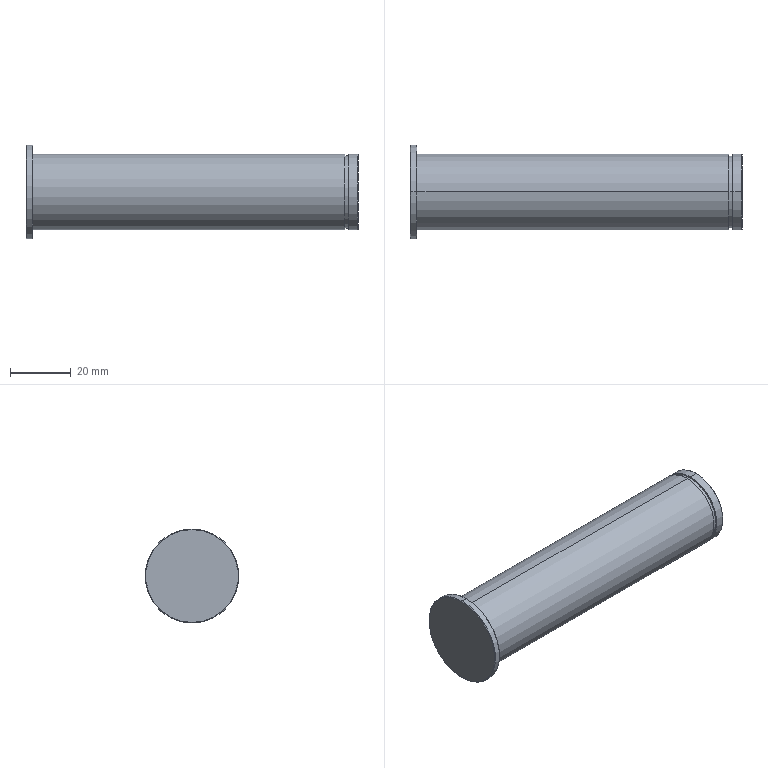Part | STEP file | BT2022003-01-04 Pin shaft A | 1 solid | 19 faces | box 109.5 x 31 x 31 mm | volume 54297 mm3 | cylinder 8 | cone 6 | plane 5 | commonest cylinder face diameters 25 x4 23.9 x2 31 x2
STEP:
#1=CARTESIAN_POINT('',(2.3,0.,-15.3));
#2=VERTEX_POINT('',#1);
#3=CARTESIAN_POINT('',(2.3,0.,15.3));
#4=VERTEX_POINT('',#3);
#5=CARTESIAN_POINT('',(2.3,0.,0.));
#6=DIRECTION('',(1.,0.,0.));
#7=DIRECTION('',(0.,0.,1.));
#8=AXIS2_PLACEMENT_3D('',#5,#6,#7);
#9=CIRCLE('',#8,15.3);
#10=EDGE_CURVE('',#2,#4,#9,.T.);
#11=ORIENTED_EDGE('',*,*,#10,.F.);
#12=CARTESIAN_POINT('',(2.1,0.,-15.5));
#13=VERTEX_POINT('',#12);
#14=CARTESIAN_POINT('',(2.1,0.,-15.5));
#15=DIRECTION('',(-0.7071,0.,-0.7071));
#16=VECTOR('',#15,1000.);
#17=LINE('',#14,#16);
#18=EDGE_CURVE('',#2,#13,#17,.T.);
#19=ORIENTED_EDGE('',*,*,#18,.T.);
#20=CARTESIAN_POINT('',(2.1,0.,15.5));
#21=VERTEX_POINT('',#20);
#22=CARTESIAN_POINT('',(2.1,0.,0.));
#23=DIRECTION('',(-1.,0.,0.));
#24=DIRECTION('',(0.,0.,1.));
#25=AXIS2_PLACEMENT_3D('',#22,#23,#24);
#26=CIRCLE('',#25,15.5);
#27=EDGE_CURVE('',#21,#13,#26,.T.);
#28=ORIENTED_EDGE('',*,*,#27,.F.);
#29=CARTESIAN_POINT('',(2.1,0.,15.5));
#30=DIRECTION('',(-0.7071,0.,0.7071));
#31=VECTOR('',#30,1000.);
#32=LINE('',#29,#31);
#33=EDGE_CURVE('',#4,#21,#32,.T.);
#34=ORIENTED_EDGE('',*,*,#33,.F.);
#35=EDGE_LOOP('',(#11,#19,#28,#34));
#36=FACE_OUTER_BOUND('',#35,.T.);
#37=CARTESIAN_POINT('',(2.1,0.,0.));
#38=DIRECTION('',(-1.,0.,0.));
#39=DIRECTION('',(0.,0.,1.));
#40=AXIS2_PLACEMENT_3D('',#37,#38,#39);
#41=CONICAL_SURFACE('',#40,15.5,0.7854);
#42=ADVANCED_FACE('',(#36),#41,.T.);
#43=CARTESIAN_POINT('',(0.,0.,15.3));
#44=VERTEX_POINT('',#43);
#45=CARTESIAN_POINT('',(0.,0.,-15.3));
#46=VERTEX_POINT('',#45);
#47=CARTESIAN_POINT('',(0.,0.,0.));
#48=DIRECTION('',(-1.,0.,0.));
#49=DIRECTION('',(0.,0.,-1.));
#50=AXIS2_PLACEMENT_3D('',#47,#48,#49);
#51=CIRCLE('',#50,15.3);
#52=EDGE_CURVE('',#44,#46,#51,.T.);
#53=ORIENTED_EDGE('',*,*,#52,.F.);
#54=CARTESIAN_POINT('',(0.2,0.,15.5));
#55=VERTEX_POINT('',#54);
#56=CARTESIAN_POINT('',(0.,0.,15.3));
#57=DIRECTION('',(0.7071,0.,0.7071));
#58=VECTOR('',#57,1000.);
#59=LINE('',#56,#58);
#60=EDGE_CURVE('',#44,#55,#59,.T.);
#61=ORIENTED_EDGE('',*,*,#60,.T.);
#62=CARTESIAN_POINT('',(0.2,0.,-15.5));
#63=VERTEX_POINT('',#62);
#64=CARTESIAN_POINT('',(0.2,0.,0.));
#65=DIRECTION('',(1.,0.,0.));
#66=DIRECTION('',(0.,0.,-1.));
#67=AXIS2_PLACEMENT_3D('',#64,#65,#66);
#68=CIRCLE('',#67,15.5);
#69=EDGE_CURVE('',#63,#55,#68,.T.);
#70=ORIENTED_EDGE('',*,*,#69,.F.);
#71=CARTESIAN_POINT('',(0.,0.,-15.3));
#72=DIRECTION('',(0.7071,0.,-0.7071));
#73=VECTOR('',#72,1000.);
#74=LINE('',#71,#73);
#75=EDGE_CURVE('',#46,#63,#74,.T.);
#76=ORIENTED_EDGE('',*,*,#75,.F.);
#77=EDGE_LOOP('',(#53,#61,#70,#76));
#78=FACE_OUTER_BOUND('',#77,.T.);
#79=CARTESIAN_POINT('',(0.,0.,0.));
#80=DIRECTION('',(1.,0.,0.));
#81=DIRECTION('',(0.,0.,-1.));
#82=AXIS2_PLACEMENT_3D('',#79,#80,#81);
#83=CONICAL_SURFACE('',#82,15.3,0.7854);
#84=ADVANCED_FACE('',(#78),#83,.T.);
#85=CARTESIAN_POINT('',(109.5,0.,-12.3));
#86=VERTEX_POINT('',#85);
#87=CARTESIAN_POINT('',(109.5,0.,12.3));
#88=VERTEX_POINT('',#87);
#89=CARTESIAN_POINT('',(109.5,0.,0.));
#90=DIRECTION('',(1.,0.,0.));
#91=DIRECTION('',(0.,0.,1.));
#92=AXIS2_PLACEMENT_3D('',#89,#90,#91);
#93=CIRCLE('',#92,12.3);
#94=EDGE_CURVE('',#86,#88,#93,.T.);
#95=ORIENTED_EDGE('',*,*,#94,.F.);
#96=CARTESIAN_POINT('',(109.3,0.,-12.5));
#97=VERTEX_POINT('',#96);
#98=CARTESIAN_POINT('',(109.3,0.,-12.5));
#99=DIRECTION('',(-0.7071,0.,-0.7071));
#100=VECTOR('',#99,1000.);
#101=LINE('',#98,#100);
#102=EDGE_CURVE('',#86,#97,#101,.T.);
#103=ORIENTED_EDGE('',*,*,#102,.T.);
#104=CARTESIAN_POINT('',(109.3,0.,12.5));
#105=VERTEX_POINT('',#104);
#106=CARTESIAN_POINT('',(109.3,0.,0.));
#107=DIRECTION('',(-1.,0.,0.));
#108=DIRECTION('',(0.,0.,1.));
#109=AXIS2_PLACEMENT_3D('',#106,#107,#108);
#110=CIRCLE('',#109,12.5);
#111=EDGE_CURVE('',#105,#97,#110,.T.);
#112=ORIENTED_EDGE('',*,*,#111,.F.);
#113=CARTESIAN_POINT('',(109.3,0.,12.5));
#114=DIRECTION('',(-0.7071,0.,0.7071));
#115=VECTOR('',#114,1000.);
#116=LINE('',#113,#115);
#117=EDGE_CURVE('',#88,#105,#116,.T.);
#118=ORIENTED_EDGE('',*,*,#117,.F.);
#119=EDGE_LOOP('',(#95,#103,#112,#118));
#120=FACE_OUTER_BOUND('',#119,.T.);
#121=CARTESIAN_POINT('',(109.3,0.,0.));
#122=DIRECTION('',(-1.,0.,0.));
#123=DIRECTION('',(0.,0.,1.));
#124=AXIS2_PLACEMENT_3D('',#121,#122,#123);
#125=CONICAL_SURFACE('',#124,12.5,0.7854);
#126=ADVANCED_FACE('',(#120),#125,.T.);
#127=ORIENTED_EDGE('',*,*,#111,.T.);
#128=CARTESIAN_POINT('',(106.5,0.,-12.5));
#129=VERTEX_POINT('',#128);
#130=CARTESIAN_POINT('',(0.,0.,-12.5));
#131=DIRECTION('',(-1.,0.,0.));
#132=VECTOR('',#131,1000.);
#133=LINE('',#130,#132);
#134=EDGE_CURVE('',#97,#129,#133,.T.);
#135=ORIENTED_EDGE('',*,*,#134,.T.);
#136=CARTESIAN_POINT('',(106.5,0.,12.5));
#137=VERTEX_POINT('',#136);
#138=CARTESIAN_POINT('',(106.5,0.,0.));
#139=DIRECTION('',(-1.,0.,0.));
#140=DIRECTION('',(0.,0.,1.));
#141=AXIS2_PLACEMENT_3D('',#138,#139,#140);
#142=CIRCLE('',#141,12.5);
#143=EDGE_CURVE('',#137,#129,#142,.T.);
#144=ORIENTED_EDGE('',*,*,#143,.F.);
#145=CARTESIAN_POINT('',(0.,0.,12.5));
#146=DIRECTION('',(-1.,0.,0.));
#147=VECTOR('',#146,1000.);
#148=LINE('',#145,#147);
#149=EDGE_CURVE('',#105,#137,#148,.T.);
#150=ORIENTED_EDGE('',*,*,#149,.F.);
#151=EDGE_LOOP('',(#127,#135,#144,#150));
#152=FACE_OUTER_BOUND('',#151,.T.);
#153=CARTESIAN_POINT('',(0.,0.,0.));
#154=DIRECTION('',(-1.,0.,0.));
#155=DIRECTION('',(0.,0.,1.));
#156=AXIS2_PLACEMENT_3D('',#153,#154,#155);
#157=CYLINDRICAL_SURFACE('',#156,12.5);
#158=ADVANCED_FACE('',(#152),#157,.T.);
#159=CARTESIAN_POINT('',(106.5,0.,11.95));
#160=VERTEX_POINT('',#159);
#161=CARTESIAN_POINT('',(106.5,0.,-11.95));
#162=VERTEX_POINT('',#161);
#163=CARTESIAN_POINT('',(106.5,0.,0.));
#164=DIRECTION('',(-1.,0.,0.));
#165=DIRECTION('',(0.,0.,1.));
#166=AXIS2_PLACEMENT_3D('',#163,#164,#165);
#167=CIRCLE('',#166,11.95);
#168=EDGE_CURVE('',#160,#162,#167,.T.);
#169=ORIENTED_EDGE('',*,*,#168,.T.);
#170=CARTESIAN_POINT('',(105.2,0.,-11.95));
#171=VERTEX_POINT('',#170);
#172=CARTESIAN_POINT('',(0.,0.,-11.95));
#173=DIRECTION('',(-1.,0.,0.));
#174=VECTOR('',#173,1000.);
#175=LINE('',#172,#174);
#176=EDGE_CURVE('',#162,#171,#175,.T.);
#177=ORIENTED_EDGE('',*,*,#176,.T.);
#178=CARTESIAN_POINT('',(105.2,0.,11.95));
#179=VERTEX_POINT('',#178);
#180=CARTESIAN_POINT('',(105.2,0.,0.));
#181=DIRECTION('',(-1.,0.,0.));
#182=DIRECTION('',(0.,0.,1.));
#183=AXIS2_PLACEMENT_3D('',#180,#181,#182);
#184=CIRCLE('',#183,11.95);
#185=EDGE_CURVE('',#179,#171,#184,.T.);
#186=ORIENTED_EDGE('',*,*,#185,.F.);
#187=CARTESIAN_POINT('',(0.,0.,11.95));
#188=DIRECTION('',(-1.,0.,0.));
#189=VECTOR('',#188,1000.);
#190=LINE('',#187,#189);
#191=EDGE_CURVE('',#160,#179,#190,.T.);
#192=ORIENTED_EDGE('',*,*,#191,.F.);
#193=EDGE_LOOP('',(#169,#177,#186,#192));
#194=FACE_OUTER_BOUND('',#193,.T.);
#195=CARTESIAN_POINT('',(0.,0.,0.));
#196=DIRECTION('',(-1.,0.,0.));
#197=DIRECTION('',(0.,0.,1.));
#198=AXIS2_PLACEMENT_3D('',#195,#196,#197);
#199=CYLINDRICAL_SURFACE('',#198,11.95);
#200=ADVANCED_FACE('',(#194),#199,.T.);
#201=CARTESIAN_POINT('',(105.2,0.,12.5));
#202=VERTEX_POINT('',#201);
#203=CARTESIAN_POINT('',(105.2,0.,-12.5));
#204=VERTEX_POINT('',#203);
#205=CARTESIAN_POINT('',(105.2,0.,0.));
#206=DIRECTION('',(-1.,0.,0.));
#207=DIRECTION('',(0.,0.,1.));
#208=AXIS2_PLACEMENT_3D('',#205,#206,#207);
#209=CIRCLE('',#208,12.5);
#210=EDGE_CURVE('',#202,#204,#209,.T.);
#211=ORIENTED_EDGE('',*,*,#210,.T.);
#212=CARTESIAN_POINT('',(2.3,0.,-12.5));
#213=VERTEX_POINT('',#212);
#214=CARTESIAN_POINT('',(0.,0.,-12.5));
#215=DIRECTION('',(-1.,0.,0.));
#216=VECTOR('',#215,1000.);
#217=LINE('',#214,#216);
#218=EDGE_CURVE('',#204,#213,#217,.T.);
#219=ORIENTED_EDGE('',*,*,#218,.T.);
#220=CARTESIAN_POINT('',(2.3,0.,12.5));
#221=VERTEX_POINT('',#220);
#222=CARTESIAN_POINT('',(2.3,0.,0.));
#223=DIRECTION('',(-1.,0.,0.));
#224=DIRECTION('',(0.,0.,1.));
#225=AXIS2_PLACEMENT_3D('',#222,#223,#224);
#226=CIRCLE('',#225,12.5);
#227=EDGE_CURVE('',#221,#213,#226,.T.);
#228=ORIENTED_EDGE('',*,*,#227,.F.);
#229=CARTESIAN_POINT('',(0.,0.,12.5));
#230=DIRECTION('',(-1.,0.,0.));
#231=VECTOR('',#230,1000.);
#232=LINE('',#229,#231);
#233=EDGE_CURVE('',#202,#221,#232,.T.);
#234=ORIENTED_EDGE('',*,*,#233,.F.);
#235=EDGE_LOOP('',(#211,#219,#228,#234));
#236=FACE_OUTER_BOUND('',#235,.T.);
#237=CARTESIAN_POINT('',(0.,0.,0.));
#238=DIRECTION('',(-1.,0.,0.));
#239=DIRECTION('',(0.,0.,1.));
#240=AXIS2_PLACEMENT_3D('',#237,#238,#239);
#241=CYLINDRICAL_SURFACE('',#240,12.5);
#242=ADVANCED_FACE('',(#236),#241,.T.);
#243=ORIENTED_EDGE('',*,*,#27,.T.);
#244=CARTESIAN_POINT('',(0.,0.,-15.5));
#245=DIRECTION('',(-1.,0.,0.));
#246=VECTOR('',#245,1000.);
#247=LINE('',#244,#246);
#248=EDGE_CURVE('',#13,#63,#247,.T.);
#249=ORIENTED_EDGE('',*,*,#248,.T.);
#250=ORIENTED_EDGE('',*,*,#69,.T.);
#251=CARTESIAN_POINT('',(0.,0.,15.5));
#252=DIRECTION('',(-1.,0.,0.));
#253=VECTOR('',#252,1000.);
#254=LINE('',#251,#253);
#255=EDGE_CURVE('',#21,#55,#254,.T.);
#256=ORIENTED_EDGE('',*,*,#255,.F.);
#257=EDGE_LOOP('',(#243,#249,#250,#256));
#258=FACE_OUTER_BOUND('',#257,.T.);
#259=CARTESIAN_POINT('',(0.,0.,0.));
#260=DIRECTION('',(-1.,0.,0.));
#261=DIRECTION('',(0.,0.,1.));
#262=AXIS2_PLACEMENT_3D('',#259,#260,#261);
#263=CYLINDRICAL_SURFACE('',#262,15.5);
#264=ADVANCED_FACE('',(#258),#263,.T.);
#265=CARTESIAN_POINT('',(0.,0.,0.));
#266=DIRECTION('',(-1.,0.,0.));
#267=DIRECTION('',(0.,0.,-1.));
#268=AXIS2_PLACEMENT_3D('',#265,#266,#267);
#269=CIRCLE('',#268,15.3);
#270=EDGE_CURVE('',#46,#44,#269,.T.);
#271=ORIENTED_EDGE('',*,*,#270,.T.);
#272=ORIENTED_EDGE('',*,*,#52,.T.);
#273=EDGE_LOOP('',(#271,#272));
#274=FACE_OUTER_BOUND('',#273,.T.);
#275=CARTESIAN_POINT('',(0.,0.,0.));
#276=DIRECTION('',(1.,0.,0.));
#277=DIRECTION('',(0.,0.,-1.));
#278=AXIS2_PLACEMENT_3D('',#275,#276,#277);
#279=PLANE('',#278);
#280=ADVANCED_FACE('',(#274),#279,.F.);
#281=ORIENTED_EDGE('',*,*,#248,.F.);
#282=CARTESIAN_POINT('',(2.1,0.,0.));
#283=DIRECTION('',(-1.,0.,0.));
#284=DIRECTION('',(0.,0.,1.));
#285=AXIS2_PLACEMENT_3D('',#282,#283,#284);
#286=CIRCLE('',#285,15.5);
#287=EDGE_CURVE('',#13,#21,#286,.T.);
#288=ORIENTED_EDGE('',*,*,#287,.T.);
#289=ORIENTED_EDGE('',*,*,#255,.T.);
#290=CARTESIAN_POINT('',(0.2,0.,0.));
#291=DIRECTION('',(1.,0.,0.));
#292=DIRECTION('',(0.,0.,-1.));
#293=AXIS2_PLACEMENT_3D('',#290,#291,#292);
#294=CIRCLE('',#293,15.5);
#295=EDGE_CURVE('',#55,#63,#294,.T.);
#296=ORIENTED_EDGE('',*,*,#295,.T.);
#297=EDGE_LOOP('',(#281,#288,#289,#296));
#298=FACE_OUTER_BOUND('',#297,.T.);
#299=CARTESIAN_POINT('',(0.,0.,0.));
#300=DIRECTION('',(-1.,0.,0.));
#301=DIRECTION('',(0.,0.,1.));
#302=AXIS2_PLACEMENT_3D('',#299,#300,#301);
#303=CYLINDRICAL_SURFACE('',#302,15.5);
#304=ADVANCED_FACE('',(#298),#303,.T.);
#305=CARTESIAN_POINT('',(2.3,0.,0.));
#306=DIRECTION('',(1.,0.,0.));
#307=DIRECTION('',(0.,0.,1.));
#308=AXIS2_PLACEMENT_3D('',#305,#306,#307);
#309=CIRCLE('',#308,15.3);
#310=EDGE_CURVE('',#4,#2,#309,.T.);
#311=ORIENTED_EDGE('',*,*,#310,.T.);
#312=ORIENTED_EDGE('',*,*,#10,.T.);
#313=EDGE_LOOP('',(#311,#312));
#314=FACE_OUTER_BOUND('',#313,.T.);
#315=ORIENTED_EDGE('',*,*,#227,.T.);
#316=CARTESIAN_POINT('',(2.3,0.,0.));
#317=DIRECTION('',(-1.,0.,0.));
#318=DIRECTION('',(0.,0.,1.));
#319=AXIS2_PLACEMENT_3D('',#316,#317,#318);
#320=CIRCLE('',#319,12.5);
#321=EDGE_CURVE('',#213,#221,#320,.T.);
#322=ORIENTED_EDGE('',*,*,#321,.T.);
#323=EDGE_LOOP('',(#315,#322));
#324=FACE_BOUND('',#323,.T.);
#325=CARTESIAN_POINT('',(2.3,15.5,0.));
#326=DIRECTION('',(-1.,0.,0.));
#327=DIRECTION('',(0.,0.,1.));
#328=AXIS2_PLACEMENT_3D('',#325,#326,#327);
#329=PLANE('',#328);
#330=ADVANCED_FACE('',(#314,#324),#329,.F.);
#331=ORIENTED_EDGE('',*,*,#218,.F.);
#332=CARTESIAN_POINT('',(105.2,0.,0.));
#333=DIRECTION('',(-1.,0.,0.));
#334=DIRECTION('',(0.,0.,1.));
#335=AXIS2_PLACEMENT_3D('',#332,#333,#334);
#336=CIRCLE('',#335,12.5);
#337=EDGE_CURVE('',#204,#202,#336,.T.);
#338=ORIENTED_EDGE('',*,*,#337,.T.);
#339=ORIENTED_EDGE('',*,*,#233,.T.);
#340=ORIENTED_EDGE('',*,*,#321,.F.);
#341=EDGE_LOOP('',(#331,#338,#339,#340));
#342=FACE_OUTER_BOUND('',#341,.T.);
#343=CARTESIAN_POINT('',(0.,0.,0.));
#344=DIRECTION('',(-1.,0.,0.));
#345=DIRECTION('',(0.,0.,1.));
#346=AXIS2_PLACEMENT_3D('',#343,#344,#345);
#347=CYLINDRICAL_SURFACE('',#346,12.5);
#348=ADVANCED_FACE('',(#342),#347,.T.);
#349=ORIENTED_EDGE('',*,*,#210,.F.);
#350=ORIENTED_EDGE('',*,*,#337,.F.);
#351=EDGE_LOOP('',(#349,#350));
#352=FACE_OUTER_BOUND('',#351,.T.);
#353=ORIENTED_EDGE('',*,*,#185,.T.);
#354=CARTESIAN_POINT('',(105.2,0.,0.));
#355=DIRECTION('',(-1.,0.,0.));
#356=DIRECTION('',(0.,0.,1.));
#357=AXIS2_PLACEMENT_3D('',#354,#355,#356);
#358=CIRCLE('',#357,11.95);
#359=EDGE_CURVE('',#171,#179,#358,.T.);
#360=ORIENTED_EDGE('',*,*,#359,.T.);
#361=EDGE_LOOP('',(#353,#360));
#362=FACE_BOUND('',#361,.T.);
#363=CARTESIAN_POINT('',(105.2,12.5,0.));
#364=DIRECTION('',(-1.,0.,0.));
#365=DIRECTION('',(0.,0.,1.));
#366=AXIS2_PLACEMENT_3D('',#363,#364,#365);
#367=PLANE('',#366);
#368=ADVANCED_FACE('',(#352,#362),#367,.F.);
#369=ORIENTED_EDGE('',*,*,#176,.F.);
#370=CARTESIAN_POINT('',(106.5,0.,0.));
#371=DIRECTION('',(-1.,0.,0.));
#372=DIRECTION('',(0.,0.,1.));
#373=AXIS2_PLACEMENT_3D('',#370,#371,#372);
#374=CIRCLE('',#373,11.95);
#375=EDGE_CURVE('',#162,#160,#374,.T.);
#376=ORIENTED_EDGE('',*,*,#375,.T.);
#377=ORIENTED_EDGE('',*,*,#191,.T.);
#378=ORIENTED_EDGE('',*,*,#359,.F.);
#379=EDGE_LOOP('',(#369,#376,#377,#378));
#380=FACE_OUTER_BOUND('',#379,.T.);
#381=CARTESIAN_POINT('',(0.,0.,0.));
#382=DIRECTION('',(-1.,0.,0.));
#383=DIRECTION('',(0.,0.,1.));
#384=AXIS2_PLACEMENT_3D('',#381,#382,#383);
#385=CYLINDRICAL_SURFACE('',#384,11.95);
#386=ADVANCED_FACE('',(#380),#385,.T.);
#387=ORIENTED_EDGE('',*,*,#168,.F.);
#388=ORIENTED_EDGE('',*,*,#375,.F.);
#389=EDGE_LOOP('',(#387,#388));
#390=FACE_BOUND('',#389,.T.);
#391=ORIENTED_EDGE('',*,*,#143,.T.);
#392=CARTESIAN_POINT('',(106.5,0.,0.));
#393=DIRECTION('',(-1.,0.,0.));
#394=DIRECTION('',(0.,0.,1.));
#395=AXIS2_PLACEMENT_3D('',#392,#393,#394);
#396=CIRCLE('',#395,12.5);
#397=EDGE_CURVE('',#129,#137,#396,.T.);
#398=ORIENTED_EDGE('',*,*,#397,.T.);
#399=EDGE_LOOP('',(#391,#398));
#400=FACE_OUTER_BOUND('',#399,.T.);
#401=CARTESIAN_POINT('',(106.5,11.95,0.));
#402=DIRECTION('',(1.,0.,0.));
#403=DIRECTION('',(0.,0.,-1.));
#404=AXIS2_PLACEMENT_3D('',#401,#402,#403);
#405=PLANE('',#404);
#406=ADVANCED_FACE('',(#390,#400),#405,.F.);
#407=ORIENTED_EDGE('',*,*,#134,.F.);
#408=CARTESIAN_POINT('',(109.3,0.,0.));
#409=DIRECTION('',(-1.,0.,0.));
#410=DIRECTION('',(0.,0.,1.));
#411=AXIS2_PLACEMENT_3D('',#408,#409,#410);
#412=CIRCLE('',#411,12.5);
#413=EDGE_CURVE('',#97,#105,#412,.T.);
#414=ORIENTED_EDGE('',*,*,#413,.T.);
#415=ORIENTED_EDGE('',*,*,#149,.T.);
#416=ORIENTED_EDGE('',*,*,#397,.F.);
#417=EDGE_LOOP('',(#407,#414,#415,#416));
#418=FACE_OUTER_BOUND('',#417,.T.);
#419=CARTESIAN_POINT('',(0.,0.,0.));
#420=DIRECTION('',(-1.,0.,0.));
#421=DIRECTION('',(0.,0.,1.));
#422=AXIS2_PLACEMENT_3D('',#419,#420,#421);
#423=CYLINDRICAL_SURFACE('',#422,12.5);
#424=ADVANCED_FACE('',(#418),#423,.T.);
#425=CARTESIAN_POINT('',(109.5,0.,0.));
#426=DIRECTION('',(1.,0.,0.));
#427=DIRECTION('',(0.,0.,1.));
#428=AXIS2_PLACEMENT_3D('',#425,#426,#427);
#429=CIRCLE('',#428,12.3);
#430=EDGE_CURVE('',#88,#86,#429,.T.);
#431=ORIENTED_EDGE('',*,*,#430,.T.);
#432=ORIENTED_EDGE('',*,*,#94,.T.);
#433=EDGE_LOOP('',(#431,#432));
#434=FACE_OUTER_BOUND('',#433,.T.);
#435=CARTESIAN_POINT('',(109.5,12.5,0.));
#436=DIRECTION('',(-1.,0.,0.));
#437=DIRECTION('',(0.,0.,1.));
#438=AXIS2_PLACEMENT_3D('',#435,#436,#437);
#439=PLANE('',#438);
#440=ADVANCED_FACE('',(#434),#439,.F.);
#441=ORIENTED_EDGE('',*,*,#102,.F.);
#442=ORIENTED_EDGE('',*,*,#430,.F.);
#443=ORIENTED_EDGE('',*,*,#117,.T.);
#444=ORIENTED_EDGE('',*,*,#413,.F.);
#445=EDGE_LOOP('',(#441,#442,#443,#444));
#446=FACE_OUTER_BOUND('',#445,.T.);
#447=CARTESIAN_POINT('',(109.3,0.,0.));
#448=DIRECTION('',(-1.,0.,0.));
#449=DIRECTION('',(0.,0.,1.));
#450=AXIS2_PLACEMENT_3D('',#447,#448,#449);
#451=CONICAL_SURFACE('',#450,12.5,0.7854);
#452=ADVANCED_FACE('',(#446),#451,.T.);
#453=ORIENTED_EDGE('',*,*,#60,.F.);
#454=ORIENTED_EDGE('',*,*,#270,.F.);
#455=ORIENTED_EDGE('',*,*,#75,.T.);
#456=ORIENTED_EDGE('',*,*,#295,.F.);
#457=EDGE_LOOP('',(#453,#454,#455,#456));
#458=FACE_OUTER_BOUND('',#457,.T.);
#459=CARTESIAN_POINT('',(0.,0.,0.));
#460=DIRECTION('',(1.,0.,0.));
#461=DIRECTION('',(0.,0.,-1.));
#462=AXIS2_PLACEMENT_3D('',#459,#460,#461);
#463=CONICAL_SURFACE('',#462,15.3,0.7854);
#464=ADVANCED_FACE('',(#458),#463,.T.);
#465=ORIENTED_EDGE('',*,*,#18,.F.);
#466=ORIENTED_EDGE('',*,*,#310,.F.);
#467=ORIENTED_EDGE('',*,*,#33,.T.);
#468=ORIENTED_EDGE('',*,*,#287,.F.);
#469=EDGE_LOOP('',(#465,#466,#467,#468));
#470=FACE_OUTER_BOUND('',#469,.T.);
#471=CARTESIAN_POINT('',(2.1,0.,0.));
#472=DIRECTION('',(-1.,0.,0.));
#473=DIRECTION('',(0.,0.,1.));
#474=AXIS2_PLACEMENT_3D('',#471,#472,#473);
#475=CONICAL_SURFACE('',#474,15.5,0.7854);
#476=ADVANCED_FACE('',(#470),#475,.T.);
#477=CLOSED_SHELL('',(#42,#84,#126,#158,#200,#242,#264,#280,#304,#330,#348,#368,#386,#406,#424,#440,#452,#464,#476));
#478=MANIFOLD_SOLID_BREP('',#477);
#479=CARTESIAN_POINT('',(0.,0.,0.));
#480=DIRECTION('',(0.,0.,1.));
#481=DIRECTION('',(1.,0.,0.));
#482=AXIS2_PLACEMENT_3D('',#479,#480,#481);
#483=(LENGTH_UNIT()NAMED_UNIT(*)SI_UNIT(.MILLI.,.METRE.));
#484=UNCERTAINTY_MEASURE_WITH_UNIT(LENGTH_MEASURE(0.00001),#483,'','');
#485=(NAMED_UNIT(*)PLANE_ANGLE_UNIT()SI_UNIT($,.RADIAN.));
#486=(NAMED_UNIT(*)SI_UNIT($,.STERADIAN.)SOLID_ANGLE_UNIT());
#487=(GEOMETRIC_REPRESENTATION_CONTEXT(3)GLOBAL_UNCERTAINTY_ASSIGNED_CONTEXT((#484))GLOBAL_UNIT_ASSIGNED_CONTEXT((#483,#485,#486))REPRESENTATION_CONTEXT('',''));
#488=ADVANCED_BREP_SHAPE_REPRESENTATION('',(#478,#482),#487);